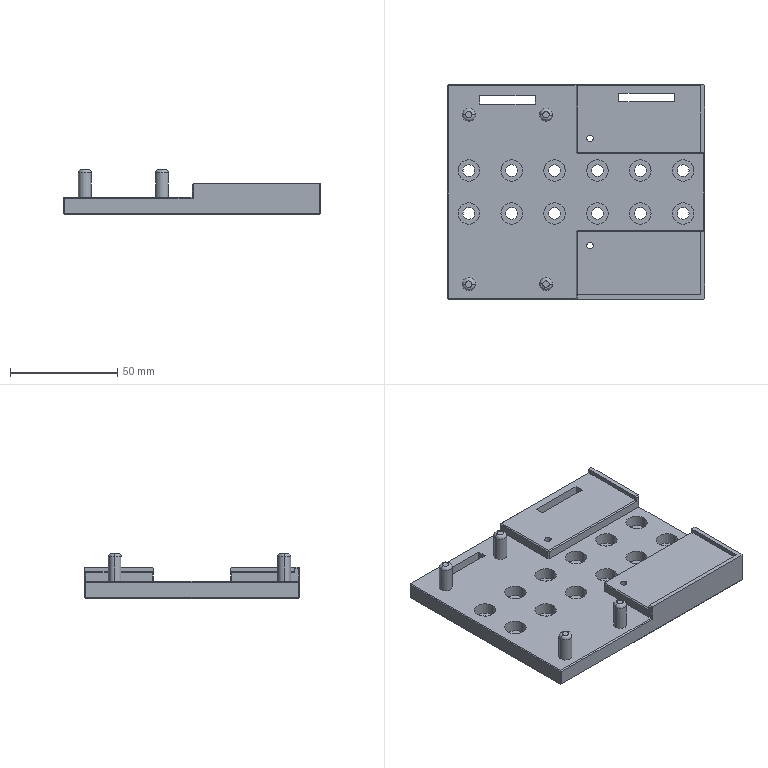Part | SolidWorks | features BaseBody 1 | 1 solid | 146 faces | box 120 x 100 x 21 mm | volume 106763 mm3 | plane 70 | cylinder 64 | cone 4 | spline 4 | torus 4 | commonest cylinder face diameters 5.5 x24 10 x24 6 x8 3 x4 3.3 x4